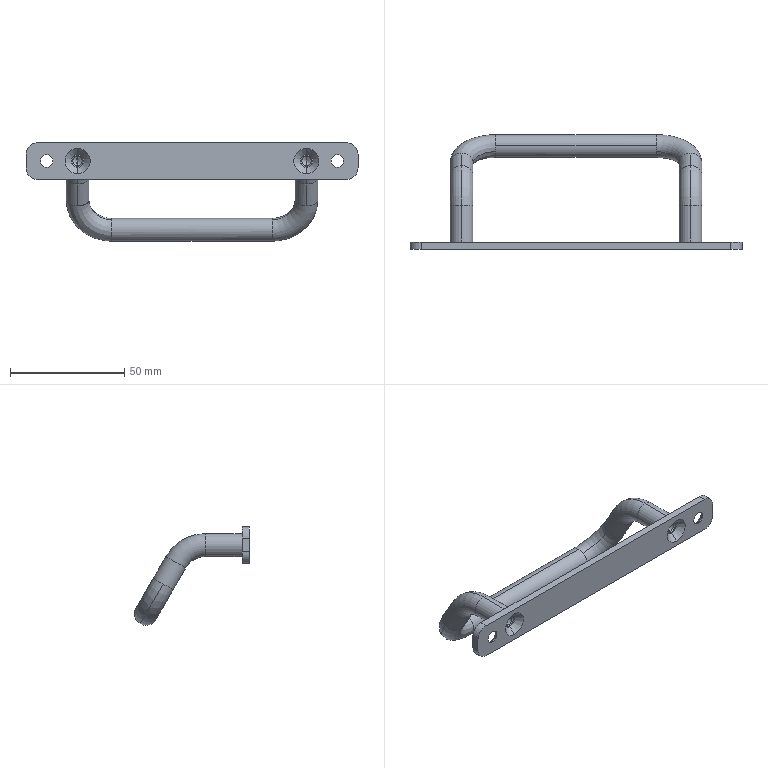Part | SolidWorks | 2 solids | 65 faces | box 145 x 50.2 x 43 mm | volume 22171 mm3 | cylinder 26 | cone 16 | plane 15 | torus 6 | spline 2 | commonest cylinder face diameters 10 x10 5.5 x8 4.134 x4 9.998 x4